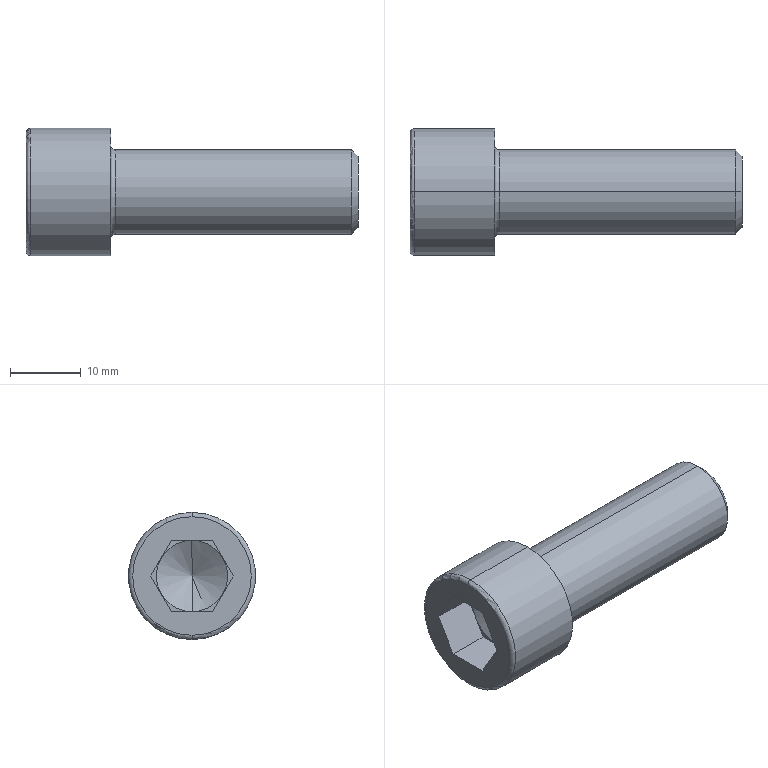Part | STEP file | socket head cap screw_iso_ISO 4762 M12 x 35 - 35N | 1 solid | 27 faces | box 47 x 18 x 18 mm | volume 6384 mm3 | plane 15 | cone 4 | torus 4 | cylinder 4 | commonest cylinder face diameters 12 x2 18 x2
STEP:
#1=CARTESIAN_POINT('',(8.92,0.,0.));
#2=VERTEX_POINT('',#1);
#3=CARTESIAN_POINT('',(6.,0.,5.057));
#4=VERTEX_POINT('',#3);
#5=CARTESIAN_POINT('',(6.,0.,5.058));
#6=DIRECTION('',(-0.5,0.,0.866));
#7=VECTOR('',#6,1000.);
#8=LINE('',#5,#7);
#9=EDGE_CURVE('',#2,#4,#8,.T.);
#10=ORIENTED_EDGE('',*,*,#9,.F.);
#11=CARTESIAN_POINT('',(6.,0.,-5.058));
#12=VERTEX_POINT('',#11);
#13=CARTESIAN_POINT('',(6.,0.,-5.058));
#14=DIRECTION('',(-0.5,0.,-0.866));
#15=VECTOR('',#14,1000.);
#16=LINE('',#13,#15);
#17=EDGE_CURVE('',#2,#12,#16,.T.);
#18=ORIENTED_EDGE('',*,*,#17,.T.);
#19=CARTESIAN_POINT('',(6.,-4.38,-2.529));
#20=VERTEX_POINT('',#19);
#21=CARTESIAN_POINT('',(6.,0.,0.));
#22=DIRECTION('',(-1.,0.,0.));
#23=DIRECTION('',(0.,0.,1.));
#24=AXIS2_PLACEMENT_3D('',#21,#22,#23);
#25=CIRCLE('',#24,5.058);
#26=EDGE_CURVE('',#12,#20,#25,.T.);
#27=ORIENTED_EDGE('',*,*,#26,.T.);
#28=CARTESIAN_POINT('',(6.,-4.38,2.529));
#29=VERTEX_POINT('',#28);
#30=CARTESIAN_POINT('',(6.,0.,0.));
#31=DIRECTION('',(-1.,0.,0.));
#32=DIRECTION('',(0.,0.,1.));
#33=AXIS2_PLACEMENT_3D('',#30,#31,#32);
#34=CIRCLE('',#33,5.058);
#35=EDGE_CURVE('',#20,#29,#34,.T.);
#36=ORIENTED_EDGE('',*,*,#35,.T.);
#37=CARTESIAN_POINT('',(6.,0.,0.));
#38=DIRECTION('',(-1.,0.,0.));
#39=DIRECTION('',(0.,0.,1.));
#40=AXIS2_PLACEMENT_3D('',#37,#38,#39);
#41=CIRCLE('',#40,5.058);
#42=EDGE_CURVE('',#29,#4,#41,.T.);
#43=ORIENTED_EDGE('',*,*,#42,.T.);
#44=EDGE_LOOP('',(#10,#18,#27,#36,#43));
#45=FACE_OUTER_BOUND('',#44,.T.);
#46=CARTESIAN_POINT('',(6.,0.,0.));
#47=DIRECTION('',(-1.,0.,0.));
#48=DIRECTION('',(0.,0.,1.));
#49=AXIS2_PLACEMENT_3D('',#46,#47,#48);
#50=CONICAL_SURFACE('',#49,5.058,1.047);
#51=ADVANCED_FACE('',(#45),#50,.F.);
#52=CARTESIAN_POINT('',(0.6,0.,-9.));
#53=VERTEX_POINT('',#52);
#54=CARTESIAN_POINT('',(0.6,0.,9.));
#55=VERTEX_POINT('',#54);
#56=CARTESIAN_POINT('',(0.6,0.,0.));
#57=DIRECTION('',(1.,0.,0.));
#58=DIRECTION('',(0.,0.,1.));
#59=AXIS2_PLACEMENT_3D('',#56,#57,#58);
#60=CIRCLE('',#59,9.);
#61=EDGE_CURVE('',#53,#55,#60,.T.);
#62=ORIENTED_EDGE('',*,*,#61,.F.);
#63=CARTESIAN_POINT('',(0.,0.,-8.4));
#64=VERTEX_POINT('',#63);
#65=CARTESIAN_POINT('',(0.6,0.,-8.4));
#66=DIRECTION('',(0.,1.,0.));
#67=DIRECTION('',(0.,0.,1.));
#68=AXIS2_PLACEMENT_3D('',#65,#66,#67);
#69=CIRCLE('',#68,0.6);
#70=EDGE_CURVE('',#53,#64,#69,.T.);
#71=ORIENTED_EDGE('',*,*,#70,.T.);
#72=CARTESIAN_POINT('',(0.,0.,8.4));
#73=VERTEX_POINT('',#72);
#74=CARTESIAN_POINT('',(0.,0.,0.));
#75=DIRECTION('',(-1.,0.,0.));
#76=DIRECTION('',(0.,0.,1.));
#77=AXIS2_PLACEMENT_3D('',#74,#75,#76);
#78=CIRCLE('',#77,8.4);
#79=EDGE_CURVE('',#73,#64,#78,.T.);
#80=ORIENTED_EDGE('',*,*,#79,.F.);
#81=CARTESIAN_POINT('',(0.6,0.,8.4));
#82=DIRECTION('',(0.,-1.,0.));
#83=DIRECTION('',(0.,0.,-1.));
#84=AXIS2_PLACEMENT_3D('',#81,#82,#83);
#85=CIRCLE('',#84,0.6);
#86=EDGE_CURVE('',#55,#73,#85,.T.);
#87=ORIENTED_EDGE('',*,*,#86,.F.);
#88=EDGE_LOOP('',(#62,#71,#80,#87));
#89=FACE_OUTER_BOUND('',#88,.T.);
#90=CARTESIAN_POINT('',(0.6,0.,0.));
#91=DIRECTION('',(-1.,0.,0.));
#92=DIRECTION('',(0.,0.,1.));
#93=AXIS2_PLACEMENT_3D('',#90,#91,#92);
#94=TOROIDAL_SURFACE('',#93,8.4,0.6);
#95=ADVANCED_FACE('',(#89),#94,.T.);
#96=CARTESIAN_POINT('',(12.6,0.,6.));
#97=VERTEX_POINT('',#96);
#98=CARTESIAN_POINT('',(12.6,0.,-6.));
#99=VERTEX_POINT('',#98);
#100=CARTESIAN_POINT('',(12.6,0.,0.));
#101=DIRECTION('',(1.,0.,0.));
#102=DIRECTION('',(0.,0.,-1.));
#103=AXIS2_PLACEMENT_3D('',#100,#101,#102);
#104=CIRCLE('',#103,6.);
#105=EDGE_CURVE('',#97,#99,#104,.T.);
#106=ORIENTED_EDGE('',*,*,#105,.F.);
#107=CARTESIAN_POINT('',(12.,0.,6.6));
#108=VERTEX_POINT('',#107);
#109=CARTESIAN_POINT('',(12.6,0.,6.6));
#110=DIRECTION('',(0.,1.,0.));
#111=DIRECTION('',(0.,0.,1.));
#112=AXIS2_PLACEMENT_3D('',#109,#110,#111);
#113=CIRCLE('',#112,0.6);
#114=EDGE_CURVE('',#97,#108,#113,.T.);
#115=ORIENTED_EDGE('',*,*,#114,.T.);
#116=CARTESIAN_POINT('',(12.,0.,-6.6));
#117=VERTEX_POINT('',#116);
#118=CARTESIAN_POINT('',(12.,0.,0.));
#119=DIRECTION('',(-1.,0.,0.));
#120=DIRECTION('',(0.,0.,-1.));
#121=AXIS2_PLACEMENT_3D('',#118,#119,#120);
#122=CIRCLE('',#121,6.6);
#123=EDGE_CURVE('',#117,#108,#122,.T.);
#124=ORIENTED_EDGE('',*,*,#123,.F.);
#125=CARTESIAN_POINT('',(12.6,0.,-6.6));
#126=DIRECTION('',(0.,-1.,0.));
#127=DIRECTION('',(0.,0.,-1.));
#128=AXIS2_PLACEMENT_3D('',#125,#126,#127);
#129=CIRCLE('',#128,0.6);
#130=EDGE_CURVE('',#99,#117,#129,.T.);
#131=ORIENTED_EDGE('',*,*,#130,.F.);
#132=EDGE_LOOP('',(#106,#115,#124,#131));
#133=FACE_OUTER_BOUND('',#132,.T.);
#134=CARTESIAN_POINT('',(12.6,0.,0.));
#135=DIRECTION('',(1.,0.,0.));
#136=DIRECTION('',(0.,0.,-1.));
#137=AXIS2_PLACEMENT_3D('',#134,#135,#136);
#138=TOROIDAL_SURFACE('',#137,6.6,0.6);
#139=ADVANCED_FACE('',(#133),#138,.F.);
#140=CARTESIAN_POINT('',(47.,0.,5.036));
#141=VERTEX_POINT('',#140);
#142=CARTESIAN_POINT('',(47.,0.,-5.036));
#143=VERTEX_POINT('',#142);
#144=CARTESIAN_POINT('',(47.,0.,0.));
#145=DIRECTION('',(-1.,0.,0.));
#146=DIRECTION('',(0.,0.,1.));
#147=AXIS2_PLACEMENT_3D('',#144,#145,#146);
#148=CIRCLE('',#147,5.036);
#149=EDGE_CURVE('',#141,#143,#148,.T.);
#150=ORIENTED_EDGE('',*,*,#149,.T.);
#151=CARTESIAN_POINT('',(46.036,0.,-6.));
#152=VERTEX_POINT('',#151);
#153=CARTESIAN_POINT('',(47.,0.,-5.036));
#154=DIRECTION('',(-0.7071,0.,-0.7071));
#155=VECTOR('',#154,1000.);
#156=LINE('',#153,#155);
#157=EDGE_CURVE('',#143,#152,#156,.T.);
#158=ORIENTED_EDGE('',*,*,#157,.T.);
#159=CARTESIAN_POINT('',(46.036,0.,6.));
#160=VERTEX_POINT('',#159);
#161=CARTESIAN_POINT('',(46.036,0.,0.));
#162=DIRECTION('',(-1.,0.,0.));
#163=DIRECTION('',(0.,0.,1.));
#164=AXIS2_PLACEMENT_3D('',#161,#162,#163);
#165=CIRCLE('',#164,6.);
#166=EDGE_CURVE('',#160,#152,#165,.T.);
#167=ORIENTED_EDGE('',*,*,#166,.F.);
#168=CARTESIAN_POINT('',(47.,0.,5.036));
#169=DIRECTION('',(-0.7071,0.,0.7071));
#170=VECTOR('',#169,1000.);
#171=LINE('',#168,#170);
#172=EDGE_CURVE('',#141,#160,#171,.T.);
#173=ORIENTED_EDGE('',*,*,#172,.F.);
#174=EDGE_LOOP('',(#150,#158,#167,#173));
#175=FACE_OUTER_BOUND('',#174,.T.);
#176=CARTESIAN_POINT('',(47.,0.,0.));
#177=DIRECTION('',(-1.,0.,0.));
#178=DIRECTION('',(0.,0.,1.));
#179=AXIS2_PLACEMENT_3D('',#176,#177,#178);
#180=CONICAL_SURFACE('',#179,5.036,0.7854);
#181=ADVANCED_FACE('',(#175),#180,.T.);
#182=ORIENTED_EDGE('',*,*,#166,.T.);
#183=CARTESIAN_POINT('',(-31.75,0.,-6.));
#184=DIRECTION('',(-1.,0.,0.));
#185=VECTOR('',#184,1000.);
#186=LINE('',#183,#185);
#187=EDGE_CURVE('',#152,#99,#186,.T.);
#188=ORIENTED_EDGE('',*,*,#187,.T.);
#189=CARTESIAN_POINT('',(12.6,0.,0.));
#190=DIRECTION('',(1.,0.,0.));
#191=DIRECTION('',(0.,0.,-1.));
#192=AXIS2_PLACEMENT_3D('',#189,#190,#191);
#193=CIRCLE('',#192,6.);
#194=EDGE_CURVE('',#99,#97,#193,.T.);
#195=ORIENTED_EDGE('',*,*,#194,.T.);
#196=CARTESIAN_POINT('',(-31.75,0.,6.));
#197=DIRECTION('',(-1.,0.,0.));
#198=VECTOR('',#197,1000.);
#199=LINE('',#196,#198);
#200=EDGE_CURVE('',#160,#97,#199,.T.);
#201=ORIENTED_EDGE('',*,*,#200,.F.);
#202=EDGE_LOOP('',(#182,#188,#195,#201));
#203=FACE_OUTER_BOUND('',#202,.T.);
#204=CARTESIAN_POINT('',(-31.75,0.,0.));
#205=DIRECTION('',(-1.,0.,0.));
#206=DIRECTION('',(0.,0.,1.));
#207=AXIS2_PLACEMENT_3D('',#204,#205,#206);
#208=CYLINDRICAL_SURFACE('',#207,6.);
#209=ADVANCED_FACE('',(#203),#208,.T.);
#210=CARTESIAN_POINT('',(12.,0.,9.));
#211=VERTEX_POINT('',#210);
#212=CARTESIAN_POINT('',(12.,0.,-9.));
#213=VERTEX_POINT('',#212);
#214=CARTESIAN_POINT('',(12.,0.,0.));
#215=DIRECTION('',(-1.,0.,0.));
#216=DIRECTION('',(0.,0.,1.));
#217=AXIS2_PLACEMENT_3D('',#214,#215,#216);
#218=CIRCLE('',#217,9.);
#219=EDGE_CURVE('',#211,#213,#218,.T.);
#220=ORIENTED_EDGE('',*,*,#219,.T.);
#221=CARTESIAN_POINT('',(-31.75,0.,-9.));
#222=DIRECTION('',(-1.,0.,0.));
#223=VECTOR('',#222,1000.);
#224=LINE('',#221,#223);
#225=EDGE_CURVE('',#213,#53,#224,.T.);
#226=ORIENTED_EDGE('',*,*,#225,.T.);
#227=ORIENTED_EDGE('',*,*,#61,.T.);
#228=CARTESIAN_POINT('',(-31.75,0.,9.));
#229=DIRECTION('',(-1.,0.,0.));
#230=VECTOR('',#229,1000.);
#231=LINE('',#228,#230);
#232=EDGE_CURVE('',#211,#55,#231,.T.);
#233=ORIENTED_EDGE('',*,*,#232,.F.);
#234=EDGE_LOOP('',(#220,#226,#227,#233));
#235=FACE_OUTER_BOUND('',#234,.T.);
#236=CARTESIAN_POINT('',(-31.75,0.,0.));
#237=DIRECTION('',(-1.,0.,0.));
#238=DIRECTION('',(0.,0.,1.));
#239=AXIS2_PLACEMENT_3D('',#236,#237,#238);
#240=CYLINDRICAL_SURFACE('',#239,9.);
#241=ADVANCED_FACE('',(#235),#240,.T.);
#242=CARTESIAN_POINT('',(0.,5.84,0.));
#243=VERTEX_POINT('',#242);
#244=CARTESIAN_POINT('',(0.,2.92,5.057));
#245=VERTEX_POINT('',#244);
#246=CARTESIAN_POINT('',(0.,5.84,0.));
#247=DIRECTION('',(0.,-0.5,0.866));
#248=VECTOR('',#247,1000.);
#249=LINE('',#246,#248);
#250=EDGE_CURVE('',#243,#245,#249,.T.);
#251=ORIENTED_EDGE('',*,*,#250,.T.);
#252=CARTESIAN_POINT('',(0.,-2.92,5.058));
#253=VERTEX_POINT('',#252);
#254=CARTESIAN_POINT('',(0.,-2.92,5.058));
#255=DIRECTION('',(0.,1.,0.));
#256=VECTOR('',#255,1000.);
#257=LINE('',#254,#256);
#258=EDGE_CURVE('',#253,#245,#257,.T.);
#259=ORIENTED_EDGE('',*,*,#258,.F.);
#260=CARTESIAN_POINT('',(0.,-5.84,0.));
#261=VERTEX_POINT('',#260);
#262=CARTESIAN_POINT('',(0.,-2.92,5.058));
#263=DIRECTION('',(0.,-0.5,-0.866));
#264=VECTOR('',#263,1000.);
#265=LINE('',#262,#264);
#266=EDGE_CURVE('',#253,#261,#265,.T.);
#267=ORIENTED_EDGE('',*,*,#266,.T.);
#268=CARTESIAN_POINT('',(0.,-2.92,-5.057));
#269=VERTEX_POINT('',#268);
#270=CARTESIAN_POINT('',(0.,-5.84,0.));
#271=DIRECTION('',(0.,0.5,-0.866));
#272=VECTOR('',#271,1000.);
#273=LINE('',#270,#272);
#274=EDGE_CURVE('',#261,#269,#273,.T.);
#275=ORIENTED_EDGE('',*,*,#274,.T.);
#276=CARTESIAN_POINT('',(0.,2.92,-5.058));
#277=VERTEX_POINT('',#276);
#278=CARTESIAN_POINT('',(0.,2.92,-5.058));
#279=DIRECTION('',(0.,-1.,0.));
#280=VECTOR('',#279,1000.);
#281=LINE('',#278,#280);
#282=EDGE_CURVE('',#277,#269,#281,.T.);
#283=ORIENTED_EDGE('',*,*,#282,.F.);
#284=CARTESIAN_POINT('',(0.,5.84,0.));
#285=DIRECTION('',(0.,-0.5,-0.866));
#286=VECTOR('',#285,1000.);
#287=LINE('',#284,#286);
#288=EDGE_CURVE('',#243,#277,#287,.T.);
#289=ORIENTED_EDGE('',*,*,#288,.F.);
#290=EDGE_LOOP('',(#251,#259,#267,#275,#283,#289));
#291=FACE_BOUND('',#290,.T.);
#292=ORIENTED_EDGE('',*,*,#79,.T.);
#293=CARTESIAN_POINT('',(0.,0.,0.));
#294=DIRECTION('',(-1.,0.,0.));
#295=DIRECTION('',(0.,0.,1.));
#296=AXIS2_PLACEMENT_3D('',#293,#294,#295);
#297=CIRCLE('',#296,8.4);
#298=EDGE_CURVE('',#64,#73,#297,.T.);
#299=ORIENTED_EDGE('',*,*,#298,.T.);
#300=EDGE_LOOP('',(#292,#299));
#301=FACE_OUTER_BOUND('',#300,.T.);
#302=CARTESIAN_POINT('',(0.,0.,0.));
#303=DIRECTION('',(-1.,0.,0.));
#304=DIRECTION('',(0.,0.,1.));
#305=AXIS2_PLACEMENT_3D('',#302,#303,#304);
#306=PLANE('',#305);
#307=ADVANCED_FACE('',(#291,#301),#306,.T.);
#308=ORIENTED_EDGE('',*,*,#225,.F.);
#309=CARTESIAN_POINT('',(12.,0.,0.));
#310=DIRECTION('',(-1.,0.,0.));
#311=DIRECTION('',(0.,0.,1.));
#312=AXIS2_PLACEMENT_3D('',#309,#310,#311);
#313=CIRCLE('',#312,9.);
#314=EDGE_CURVE('',#213,#211,#313,.T.);
#315=ORIENTED_EDGE('',*,*,#314,.T.);
#316=ORIENTED_EDGE('',*,*,#232,.T.);
#317=CARTESIAN_POINT('',(0.6,0.,0.));
#318=DIRECTION('',(1.,0.,0.));
#319=DIRECTION('',(0.,0.,1.));
#320=AXIS2_PLACEMENT_3D('',#317,#318,#319);
#321=CIRCLE('',#320,9.);
#322=EDGE_CURVE('',#55,#53,#321,.T.);
#323=ORIENTED_EDGE('',*,*,#322,.T.);
#324=EDGE_LOOP('',(#308,#315,#316,#323));
#325=FACE_OUTER_BOUND('',#324,.T.);
#326=CARTESIAN_POINT('',(-31.75,0.,0.));
#327=DIRECTION('',(-1.,0.,0.));
#328=DIRECTION('',(0.,0.,1.));
#329=AXIS2_PLACEMENT_3D('',#326,#327,#328);
#330=CYLINDRICAL_SURFACE('',#329,9.);
#331=ADVANCED_FACE('',(#325),#330,.T.);
#332=ORIENTED_EDGE('',*,*,#123,.T.);
#333=CARTESIAN_POINT('',(12.,0.,0.));
#334=DIRECTION('',(-1.,0.,0.));
#335=DIRECTION('',(0.,0.,-1.));
#336=AXIS2_PLACEMENT_3D('',#333,#334,#335);
#337=CIRCLE('',#336,6.6);
#338=EDGE_CURVE('',#108,#117,#337,.T.);
#339=ORIENTED_EDGE('',*,*,#338,.T.);
#340=EDGE_LOOP('',(#332,#339));
#341=FACE_BOUND('',#340,.T.);
#342=ORIENTED_EDGE('',*,*,#219,.F.);
#343=ORIENTED_EDGE('',*,*,#314,.F.);
#344=EDGE_LOOP('',(#342,#343));
#345=FACE_OUTER_BOUND('',#344,.T.);
#346=CARTESIAN_POINT('',(12.,9.,0.));
#347=DIRECTION('',(1.,0.,0.));
#348=DIRECTION('',(0.,0.,-1.));
#349=AXIS2_PLACEMENT_3D('',#346,#347,#348);
#350=PLANE('',#349);
#351=ADVANCED_FACE('',(#341,#345),#350,.T.);
#352=ORIENTED_EDGE('',*,*,#187,.F.);
#353=CARTESIAN_POINT('',(46.036,0.,0.));
#354=DIRECTION('',(-1.,0.,0.));
#355=DIRECTION('',(0.,0.,1.));
#356=AXIS2_PLACEMENT_3D('',#353,#354,#355);
#357=CIRCLE('',#356,6.);
#358=EDGE_CURVE('',#152,#160,#357,.T.);
#359=ORIENTED_EDGE('',*,*,#358,.T.);
#360=ORIENTED_EDGE('',*,*,#200,.T.);
#361=ORIENTED_EDGE('',*,*,#105,.T.);
#362=EDGE_LOOP('',(#352,#359,#360,#361));
#363=FACE_OUTER_BOUND('',#362,.T.);
#364=CARTESIAN_POINT('',(-31.75,0.,0.));
#365=DIRECTION('',(-1.,0.,0.));
#366=DIRECTION('',(0.,0.,1.));
#367=AXIS2_PLACEMENT_3D('',#364,#365,#366);
#368=CYLINDRICAL_SURFACE('',#367,6.);
#369=ADVANCED_FACE('',(#363),#368,.T.);
#370=ORIENTED_EDGE('',*,*,#157,.F.);
#371=CARTESIAN_POINT('',(47.,0.,0.));
#372=DIRECTION('',(-1.,0.,0.));
#373=DIRECTION('',(0.,0.,1.));
#374=AXIS2_PLACEMENT_3D('',#371,#372,#373);
#375=CIRCLE('',#374,5.036);
#376=EDGE_CURVE('',#143,#141,#375,.T.);
#377=ORIENTED_EDGE('',*,*,#376,.T.);
#378=ORIENTED_EDGE('',*,*,#172,.T.);
#379=ORIENTED_EDGE('',*,*,#358,.F.);
#380=EDGE_LOOP('',(#370,#377,#378,#379));
#381=FACE_OUTER_BOUND('',#380,.T.);
#382=CARTESIAN_POINT('',(47.,0.,0.));
#383=DIRECTION('',(-1.,0.,0.));
#384=DIRECTION('',(0.,0.,1.));
#385=AXIS2_PLACEMENT_3D('',#382,#383,#384);
#386=CONICAL_SURFACE('',#385,5.036,0.7854);
#387=ADVANCED_FACE('',(#381),#386,.T.);
#388=ORIENTED_EDGE('',*,*,#149,.F.);
#389=ORIENTED_EDGE('',*,*,#376,.F.);
#390=EDGE_LOOP('',(#388,#389));
#391=FACE_OUTER_BOUND('',#390,.T.);
#392=CARTESIAN_POINT('',(47.,5.036,0.));
#393=DIRECTION('',(1.,0.,0.));
#394=DIRECTION('',(0.,0.,-1.));
#395=AXIS2_PLACEMENT_3D('',#392,#393,#394);
#396=PLANE('',#395);
#397=ADVANCED_FACE('',(#391),#396,.T.);
#398=ORIENTED_EDGE('',*,*,#114,.F.);
#399=ORIENTED_EDGE('',*,*,#194,.F.);
#400=ORIENTED_EDGE('',*,*,#130,.T.);
#401=ORIENTED_EDGE('',*,*,#338,.F.);
#402=EDGE_LOOP('',(#398,#399,#400,#401));
#403=FACE_OUTER_BOUND('',#402,.T.);
#404=CARTESIAN_POINT('',(12.6,0.,0.));
#405=DIRECTION('',(1.,0.,0.));
#406=DIRECTION('',(0.,0.,-1.));
#407=AXIS2_PLACEMENT_3D('',#404,#405,#406);
#408=TOROIDAL_SURFACE('',#407,6.6,0.6);
#409=ADVANCED_FACE('',(#403),#408,.F.);
#410=ORIENTED_EDGE('',*,*,#70,.F.);
#411=ORIENTED_EDGE('',*,*,#322,.F.);
#412=ORIENTED_EDGE('',*,*,#86,.T.);
#413=ORIENTED_EDGE('',*,*,#298,.F.);
#414=EDGE_LOOP('',(#410,#411,#412,#413));
#415=FACE_OUTER_BOUND('',#414,.T.);
#416=CARTESIAN_POINT('',(0.6,0.,0.));
#417=DIRECTION('',(-1.,0.,0.));
#418=DIRECTION('',(0.,0.,1.));
#419=AXIS2_PLACEMENT_3D('',#416,#417,#418);
#420=TOROIDAL_SURFACE('',#419,8.4,0.6);
#421=ADVANCED_FACE('',(#415),#420,.T.);
#422=ORIENTED_EDGE('',*,*,#250,.F.);
#423=CARTESIAN_POINT('',(6.,5.84,0.));
#424=VERTEX_POINT('',#423);
#425=CARTESIAN_POINT('',(6.,5.84,0.));
#426=DIRECTION('',(-1.,0.,0.));
#427=VECTOR('',#426,1000.);
#428=LINE('',#425,#427);
#429=EDGE_CURVE('',#424,#243,#428,.T.);
#430=ORIENTED_EDGE('',*,*,#429,.F.);
#431=CARTESIAN_POINT('',(6.,4.38,2.529));
#432=VERTEX_POINT('',#431);
#433=CARTESIAN_POINT('',(6.,5.84,0.));
#434=DIRECTION('',(0.,-0.5,0.866));
#435=VECTOR('',#434,1000.);
#436=LINE('',#433,#435);
#437=EDGE_CURVE('',#424,#432,#436,.T.);
#438=ORIENTED_EDGE('',*,*,#437,.T.);
#439=CARTESIAN_POINT('',(6.,2.92,5.057));
#440=VERTEX_POINT('',#439);
#441=CARTESIAN_POINT('',(6.,5.84,0.));
#442=DIRECTION('',(0.,-0.5,0.866));
#443=VECTOR('',#442,1000.);
#444=LINE('',#441,#443);
#445=EDGE_CURVE('',#432,#440,#444,.T.);
#446=ORIENTED_EDGE('',*,*,#445,.T.);
#447=CARTESIAN_POINT('',(6.,2.92,5.057));
#448=DIRECTION('',(-1.,0.,0.));
#449=VECTOR('',#448,1000.);
#450=LINE('',#447,#449);
#451=EDGE_CURVE('',#440,#245,#450,.T.);
#452=ORIENTED_EDGE('',*,*,#451,.T.);
#453=EDGE_LOOP('',(#422,#430,#438,#446,#452));
#454=FACE_OUTER_BOUND('',#453,.T.);
#455=CARTESIAN_POINT('',(6.,5.84,0.));
#456=DIRECTION('',(0.,-0.866,-0.5));
#457=DIRECTION('',(0.,0.5,-0.866));
#458=AXIS2_PLACEMENT_3D('',#455,#456,#457);
#459=PLANE('',#458);
#460=ADVANCED_FACE('',(#454),#459,.T.);
#461=ORIENTED_EDGE('',*,*,#258,.T.);
#462=ORIENTED_EDGE('',*,*,#451,.F.);
#463=CARTESIAN_POINT('',(6.,-2.92,5.058));
#464=DIRECTION('',(0.,1.,0.));
#465=VECTOR('',#464,1000.);
#466=LINE('',#463,#465);
#467=EDGE_CURVE('',#4,#440,#466,.T.);
#468=ORIENTED_EDGE('',*,*,#467,.F.);
#469=CARTESIAN_POINT('',(6.,-2.92,5.058));
#470=VERTEX_POINT('',#469);
#471=CARTESIAN_POINT('',(6.,-2.92,5.058));
#472=DIRECTION('',(0.,1.,0.));
#473=VECTOR('',#472,1000.);
#474=LINE('',#471,#473);
#475=EDGE_CURVE('',#470,#4,#474,.T.);
#476=ORIENTED_EDGE('',*,*,#475,.F.);
#477=CARTESIAN_POINT('',(6.,-2.92,5.058));
#478=DIRECTION('',(-1.,0.,0.));
#479=VECTOR('',#478,1000.);
#480=LINE('',#477,#479);
#481=EDGE_CURVE('',#470,#253,#480,.T.);
#482=ORIENTED_EDGE('',*,*,#481,.T.);
#483=EDGE_LOOP('',(#461,#462,#468,#476,#482));
#484=FACE_OUTER_BOUND('',#483,.T.);
#485=CARTESIAN_POINT('',(6.,-2.92,5.058));
#486=DIRECTION('',(0.,0.,1.));
#487=DIRECTION('',(0.,-1.,0.));
#488=AXIS2_PLACEMENT_3D('',#485,#486,#487);
#489=PLANE('',#488);
#490=ADVANCED_FACE('',(#484),#489,.F.);
#491=ORIENTED_EDGE('',*,*,#266,.F.);
#492=ORIENTED_EDGE('',*,*,#481,.F.);
#493=CARTESIAN_POINT('',(6.,-2.92,5.058));
#494=DIRECTION('',(0.,-0.5,-0.866));
#495=VECTOR('',#494,1000.);
#496=LINE('',#493,#495);
#497=EDGE_CURVE('',#470,#29,#496,.T.);
#498=ORIENTED_EDGE('',*,*,#497,.T.);
#499=CARTESIAN_POINT('',(6.,-5.84,0.));
#500=VERTEX_POINT('',#499);
#501=CARTESIAN_POINT('',(6.,-2.92,5.058));
#502=DIRECTION('',(0.,-0.5,-0.866));
#503=VECTOR('',#502,1000.);
#504=LINE('',#501,#503);
#505=EDGE_CURVE('',#29,#500,#504,.T.);
#506=ORIENTED_EDGE('',*,*,#505,.T.);
#507=CARTESIAN_POINT('',(6.,-5.84,0.));
#508=DIRECTION('',(-1.,0.,0.));
#509=VECTOR('',#508,1000.);
#510=LINE('',#507,#509);
#511=EDGE_CURVE('',#500,#261,#510,.T.);
#512=ORIENTED_EDGE('',*,*,#511,.T.);
#513=EDGE_LOOP('',(#491,#492,#498,#506,#512));
#514=FACE_OUTER_BOUND('',#513,.T.);
#515=CARTESIAN_POINT('',(6.,-2.92,5.058));
#516=DIRECTION('',(0.,0.866,-0.5));
#517=DIRECTION('',(0.,0.5,0.866));
#518=AXIS2_PLACEMENT_3D('',#515,#516,#517);
#519=PLANE('',#518);
#520=ADVANCED_FACE('',(#514),#519,.T.);
#521=ORIENTED_EDGE('',*,*,#274,.F.);
#522=ORIENTED_EDGE('',*,*,#511,.F.);
#523=CARTESIAN_POINT('',(6.,-5.84,0.));
#524=DIRECTION('',(0.,0.5,-0.866));
#525=VECTOR('',#524,1000.);
#526=LINE('',#523,#525);
#527=EDGE_CURVE('',#500,#20,#526,.T.);
#528=ORIENTED_EDGE('',*,*,#527,.T.);
#529=CARTESIAN_POINT('',(6.,-2.92,-5.057));
#530=VERTEX_POINT('',#529);
#531=CARTESIAN_POINT('',(6.,-5.84,0.));
#532=DIRECTION('',(0.,0.5,-0.866));
#533=VECTOR('',#532,1000.);
#534=LINE('',#531,#533);
#535=EDGE_CURVE('',#20,#530,#534,.T.);
#536=ORIENTED_EDGE('',*,*,#535,.T.);
#537=CARTESIAN_POINT('',(6.,-2.92,-5.057));
#538=DIRECTION('',(-1.,0.,0.));
#539=VECTOR('',#538,1000.);
#540=LINE('',#537,#539);
#541=EDGE_CURVE('',#530,#269,#540,.T.);
#542=ORIENTED_EDGE('',*,*,#541,.T.);
#543=EDGE_LOOP('',(#521,#522,#528,#536,#542));
#544=FACE_OUTER_BOUND('',#543,.T.);
#545=CARTESIAN_POINT('',(6.,-5.84,0.));
#546=DIRECTION('',(0.,0.866,0.5));
#547=DIRECTION('',(0.,-0.5,0.866));
#548=AXIS2_PLACEMENT_3D('',#545,#546,#547);
#549=PLANE('',#548);
#550=ADVANCED_FACE('',(#544),#549,.T.);
#551=ORIENTED_EDGE('',*,*,#282,.T.);
#552=ORIENTED_EDGE('',*,*,#541,.F.);
#553=CARTESIAN_POINT('',(6.,2.92,-5.058));
#554=DIRECTION('',(0.,-1.,0.));
#555=VECTOR('',#554,1000.);
#556=LINE('',#553,#555);
#557=EDGE_CURVE('',#12,#530,#556,.T.);
#558=ORIENTED_EDGE('',*,*,#557,.F.);
#559=CARTESIAN_POINT('',(6.,2.92,-5.058));
#560=VERTEX_POINT('',#559);
#561=CARTESIAN_POINT('',(6.,2.92,-5.058));
#562=DIRECTION('',(0.,-1.,0.));
#563=VECTOR('',#562,1000.);
#564=LINE('',#561,#563);
#565=EDGE_CURVE('',#560,#12,#564,.T.);
#566=ORIENTED_EDGE('',*,*,#565,.F.);
#567=CARTESIAN_POINT('',(6.,2.92,-5.058));
#568=DIRECTION('',(-1.,0.,0.));
#569=VECTOR('',#568,1000.);
#570=LINE('',#567,#569);
#571=EDGE_CURVE('',#560,#277,#570,.T.);
#572=ORIENTED_EDGE('',*,*,#571,.T.);
#573=EDGE_LOOP('',(#551,#552,#558,#566,#572));
#574=FACE_OUTER_BOUND('',#573,.T.);
#575=CARTESIAN_POINT('',(6.,2.92,-5.058));
#576=DIRECTION('',(0.,0.,-1.));
#577=DIRECTION('',(0.,1.,0.));
#578=AXIS2_PLACEMENT_3D('',#575,#576,#577);
#579=PLANE('',#578);
#580=ADVANCED_FACE('',(#574),#579,.F.);
#581=ORIENTED_EDGE('',*,*,#288,.T.);
#582=ORIENTED_EDGE('',*,*,#571,.F.);
#583=CARTESIAN_POINT('',(6.,4.38,-2.529));
#584=VERTEX_POINT('',#583);
#585=CARTESIAN_POINT('',(6.,5.84,0.));
#586=DIRECTION('',(0.,-0.5,-0.866));
#587=VECTOR('',#586,1000.);
#588=LINE('',#585,#587);
#589=EDGE_CURVE('',#584,#560,#588,.T.);
#590=ORIENTED_EDGE('',*,*,#589,.F.);
#591=CARTESIAN_POINT('',(6.,5.84,0.));
#592=DIRECTION('',(0.,-0.5,-0.866));
#593=VECTOR('',#592,1000.);
#594=LINE('',#591,#593);
#595=EDGE_CURVE('',#424,#584,#594,.T.);
#596=ORIENTED_EDGE('',*,*,#595,.F.);
#597=ORIENTED_EDGE('',*,*,#429,.T.);
#598=EDGE_LOOP('',(#581,#582,#590,#596,#597));
#599=FACE_OUTER_BOUND('',#598,.T.);
#600=CARTESIAN_POINT('',(6.,5.84,0.));
#601=DIRECTION('',(0.,0.866,-0.5));
#602=DIRECTION('',(0.,0.5,0.866));
#603=AXIS2_PLACEMENT_3D('',#600,#601,#602);
#604=PLANE('',#603);
#605=ADVANCED_FACE('',(#599),#604,.F.);
#606=ORIENTED_EDGE('',*,*,#557,.T.);
#607=ORIENTED_EDGE('',*,*,#535,.F.);
#608=ORIENTED_EDGE('',*,*,#26,.F.);
#609=EDGE_LOOP('',(#606,#607,#608));
#610=FACE_OUTER_BOUND('',#609,.T.);
#611=CARTESIAN_POINT('',(6.,0.,10.115));
#612=DIRECTION('',(1.,0.,0.));
#613=DIRECTION('',(0.,0.,-1.));
#614=AXIS2_PLACEMENT_3D('',#611,#612,#613);
#615=PLANE('',#614);
#616=ADVANCED_FACE('',(#610),#615,.F.);
#617=ORIENTED_EDGE('',*,*,#527,.F.);
#618=ORIENTED_EDGE('',*,*,#505,.F.);
#619=ORIENTED_EDGE('',*,*,#35,.F.);
#620=EDGE_LOOP('',(#617,#618,#619));
#621=FACE_OUTER_BOUND('',#620,.T.);
#622=CARTESIAN_POINT('',(6.,0.,10.115));
#623=DIRECTION('',(1.,0.,0.));
#624=DIRECTION('',(0.,0.,-1.));
#625=AXIS2_PLACEMENT_3D('',#622,#623,#624);
#626=PLANE('',#625);
#627=ADVANCED_FACE('',(#621),#626,.F.);
#628=ORIENTED_EDGE('',*,*,#497,.F.);
#629=ORIENTED_EDGE('',*,*,#475,.T.);
#630=ORIENTED_EDGE('',*,*,#42,.F.);
#631=EDGE_LOOP('',(#628,#629,#630));
#632=FACE_OUTER_BOUND('',#631,.T.);
#633=CARTESIAN_POINT('',(6.,0.,10.115));
#634=DIRECTION('',(1.,0.,0.));
#635=DIRECTION('',(0.,0.,-1.));
#636=AXIS2_PLACEMENT_3D('',#633,#634,#635);
#637=PLANE('',#636);
#638=ADVANCED_FACE('',(#632),#637,.F.);
#639=ORIENTED_EDGE('',*,*,#467,.T.);
#640=ORIENTED_EDGE('',*,*,#445,.F.);
#641=CARTESIAN_POINT('',(6.,0.,0.));
#642=DIRECTION('',(-1.,0.,0.));
#643=DIRECTION('',(0.,0.,1.));
#644=AXIS2_PLACEMENT_3D('',#641,#642,#643);
#645=CIRCLE('',#644,5.058);
#646=EDGE_CURVE('',#4,#432,#645,.T.);
#647=ORIENTED_EDGE('',*,*,#646,.F.);
#648=EDGE_LOOP('',(#639,#640,#647));
#649=FACE_OUTER_BOUND('',#648,.T.);
#650=CARTESIAN_POINT('',(6.,0.,10.115));
#651=DIRECTION('',(1.,0.,0.));
#652=DIRECTION('',(0.,0.,-1.));
#653=AXIS2_PLACEMENT_3D('',#650,#651,#652);
#654=PLANE('',#653);
#655=ADVANCED_FACE('',(#649),#654,.F.);
#656=ORIENTED_EDGE('',*,*,#437,.F.);
#657=ORIENTED_EDGE('',*,*,#595,.T.);
#658=CARTESIAN_POINT('',(6.,0.,0.));
#659=DIRECTION('',(-1.,0.,0.));
#660=DIRECTION('',(0.,0.,1.));
#661=AXIS2_PLACEMENT_3D('',#658,#659,#660);
#662=CIRCLE('',#661,5.058);
#663=EDGE_CURVE('',#432,#584,#662,.T.);
#664=ORIENTED_EDGE('',*,*,#663,.F.);
#665=EDGE_LOOP('',(#656,#657,#664));
#666=FACE_OUTER_BOUND('',#665,.T.);
#667=CARTESIAN_POINT('',(6.,0.,10.115));
#668=DIRECTION('',(1.,0.,0.));
#669=DIRECTION('',(0.,0.,-1.));
#670=AXIS2_PLACEMENT_3D('',#667,#668,#669);
#671=PLANE('',#670);
#672=ADVANCED_FACE('',(#666),#671,.F.);
#673=ORIENTED_EDGE('',*,*,#589,.T.);
#674=ORIENTED_EDGE('',*,*,#565,.T.);
#675=CARTESIAN_POINT('',(6.,0.,0.));
#676=DIRECTION('',(-1.,0.,0.));
#677=DIRECTION('',(0.,0.,1.));
#678=AXIS2_PLACEMENT_3D('',#675,#676,#677);
#679=CIRCLE('',#678,5.058);
#680=EDGE_CURVE('',#584,#12,#679,.T.);
#681=ORIENTED_EDGE('',*,*,#680,.F.);
#682=EDGE_LOOP('',(#673,#674,#681));
#683=FACE_OUTER_BOUND('',#682,.T.);
#684=CARTESIAN_POINT('',(6.,0.,10.115));
#685=DIRECTION('',(1.,0.,0.));
#686=DIRECTION('',(0.,0.,-1.));
#687=AXIS2_PLACEMENT_3D('',#684,#685,#686);
#688=PLANE('',#687);
#689=ADVANCED_FACE('',(#683),#688,.F.);
#690=ORIENTED_EDGE('',*,*,#17,.F.);
#691=ORIENTED_EDGE('',*,*,#9,.T.);
#692=ORIENTED_EDGE('',*,*,#646,.T.);
#693=ORIENTED_EDGE('',*,*,#663,.T.);
#694=ORIENTED_EDGE('',*,*,#680,.T.);
#695=EDGE_LOOP('',(#690,#691,#692,#693,#694));
#696=FACE_OUTER_BOUND('',#695,.T.);
#697=CARTESIAN_POINT('',(6.,0.,0.));
#698=DIRECTION('',(-1.,0.,0.));
#699=DIRECTION('',(0.,0.,1.));
#700=AXIS2_PLACEMENT_3D('',#697,#698,#699);
#701=CONICAL_SURFACE('',#700,5.058,1.047);
#702=ADVANCED_FACE('',(#696),#701,.F.);
#703=CLOSED_SHELL('',(#51,#95,#139,#181,#209,#241,#307,#331,#351,#369,#387,#397,#409,#421,#460,#490,#520,#550,#580,#605,#616,#627,#638,#655,#672,#689,#702));
#704=MANIFOLD_SOLID_BREP('',#703);
#705=CARTESIAN_POINT('',(0.,0.,0.));
#706=DIRECTION('',(0.,0.,1.));
#707=DIRECTION('',(1.,0.,0.));
#708=AXIS2_PLACEMENT_3D('',#705,#706,#707);
#709=(LENGTH_UNIT()NAMED_UNIT(*)SI_UNIT(.MILLI.,.METRE.));
#710=UNCERTAINTY_MEASURE_WITH_UNIT(LENGTH_MEASURE(0.00001),#709,'','');
#711=(NAMED_UNIT(*)PLANE_ANGLE_UNIT()SI_UNIT($,.RADIAN.));
#712=(NAMED_UNIT(*)SI_UNIT($,.STERADIAN.)SOLID_ANGLE_UNIT());
#713=(GEOMETRIC_REPRESENTATION_CONTEXT(3)GLOBAL_UNCERTAINTY_ASSIGNED_CONTEXT((#710))GLOBAL_UNIT_ASSIGNED_CONTEXT((#709,#711,#712))REPRESENTATION_CONTEXT('',''));
#714=ADVANCED_BREP_SHAPE_REPRESENTATION('',(#704,#708),#713);